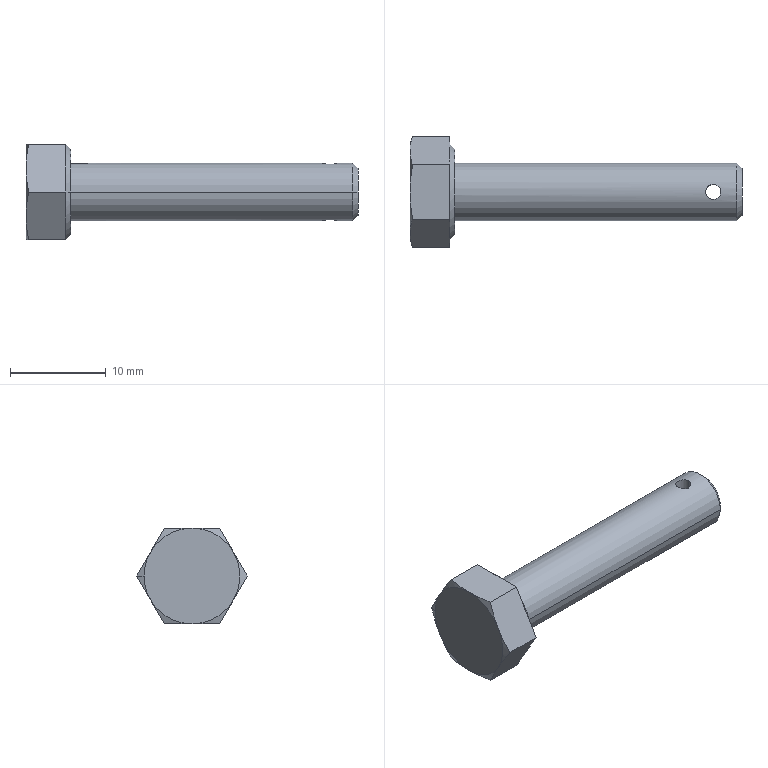Part | SolidWorks | features BaseBody 1 | 1 solid | 30 faces | box 34.65 x 11.547 x 10 mm | volume 1227 mm3 | plane 15 | cone 11 | cylinder 4 | commonest cylinder face diameters 1.6 x2 6 x2
STEP:
#1=CARTESIAN_POINT('',(30.85,0.,-3.));
#2=VERTEX_POINT('',#1);
#3=CARTESIAN_POINT('',(32.45,0.,-3.));
#4=VERTEX_POINT('',#3);
#5=CARTESIAN_POINT('',(30.85,0.,-3.));
#6=CARTESIAN_POINT('',(30.85,-0.1047,-3.));
#7=CARTESIAN_POINT('',(30.871,-0.2104,-2.994));
#8=CARTESIAN_POINT('',(30.951,-0.4032,-2.974));
#9=CARTESIAN_POINT('',(31.01,-0.4917,-2.96));
#10=CARTESIAN_POINT('',(31.232,-0.7131,-2.918));
#11=CARTESIAN_POINT('',(31.439,-0.7999,-2.891));
#12=CARTESIAN_POINT('',(31.755,-0.8,-2.891));
#13=CARTESIAN_POINT('',(31.86,-0.7789,-2.897));
#14=CARTESIAN_POINT('',(32.053,-0.6988,-2.918));
#15=CARTESIAN_POINT('',(32.142,-0.6393,-2.932));
#16=CARTESIAN_POINT('',(32.289,-0.4926,-2.96));
#17=CARTESIAN_POINT('',(32.348,-0.404,-2.974));
#18=CARTESIAN_POINT('',(32.429,-0.2113,-2.994));
#19=CARTESIAN_POINT('',(32.45,-0.1062,-3.));
#20=CARTESIAN_POINT('',(32.45,0.,-3.));
#21=B_SPLINE_CURVE_WITH_KNOTS('',3,(#5,#6,#7,#8,#9,#10,#11,#12,#13,#14,#15,#16,#17,#18,#19,#20),.UNSPECIFIED.,.F.,.F.,(4,2,2,2,2,2,2,4),(0.002513,0.002827,0.003141,0.003769,0.004083,0.004397,0.00471,0.005024),.UNSPECIFIED.);
#22=EDGE_CURVE('',#2,#4,#21,.T.);
#23=ORIENTED_EDGE('',*,*,#22,.F.);
#24=CARTESIAN_POINT('',(30.85,0.,3.));
#25=VERTEX_POINT('',#24);
#26=CARTESIAN_POINT('',(30.85,0.,-5.));
#27=DIRECTION('',(0.,0.,1.));
#28=VECTOR('',#27,1000.);
#29=LINE('',#26,#28);
#30=EDGE_CURVE('',#2,#25,#29,.T.);
#31=ORIENTED_EDGE('',*,*,#30,.T.);
#32=CARTESIAN_POINT('',(32.45,0.,3.));
#33=VERTEX_POINT('',#32);
#34=CARTESIAN_POINT('',(32.45,0.,3.));
#35=CARTESIAN_POINT('',(32.45,-0.1062,3.));
#36=CARTESIAN_POINT('',(32.429,-0.2104,2.994));
#37=CARTESIAN_POINT('',(32.348,-0.404,2.974));
#38=CARTESIAN_POINT('',(32.289,-0.4925,2.96));
#39=CARTESIAN_POINT('',(32.142,-0.6393,2.932));
#40=CARTESIAN_POINT('',(32.053,-0.6988,2.918));
#41=CARTESIAN_POINT('',(31.861,-0.7787,2.897));
#42=CARTESIAN_POINT('',(31.755,-0.8,2.891));
#43=CARTESIAN_POINT('',(31.545,-0.8,2.891));
#44=CARTESIAN_POINT('',(31.44,-0.7792,2.897));
#45=CARTESIAN_POINT('',(31.246,-0.6985,2.918));
#46=CARTESIAN_POINT('',(31.158,-0.6396,2.932));
#47=CARTESIAN_POINT('',(31.01,-0.4915,2.96));
#48=CARTESIAN_POINT('',(30.951,-0.4033,2.974));
#49=CARTESIAN_POINT('',(30.871,-0.2102,2.994));
#50=CARTESIAN_POINT('',(30.85,-0.1047,3.));
#51=CARTESIAN_POINT('',(30.85,0.,3.));
#52=B_SPLINE_CURVE_WITH_KNOTS('',3,(#34,#35,#36,#37,#38,#39,#40,#41,#42,#43,#44,#45,#46,#47,#48,#49,#50,#51),.UNSPECIFIED.,.F.,.F.,(4,2,2,2,2,2,2,2,4),(0.,0.0003141,0.0006281,0.0009422,0.001256,0.00157,0.001884,0.002199,0.002513),.UNSPECIFIED.);
#53=EDGE_CURVE('',#33,#25,#52,.T.);
#54=ORIENTED_EDGE('',*,*,#53,.F.);
#55=CARTESIAN_POINT('',(32.45,0.,-5.));
#56=DIRECTION('',(0.,0.,1.));
#57=VECTOR('',#56,1000.);
#58=LINE('',#55,#57);
#59=EDGE_CURVE('',#4,#33,#58,.T.);
#60=ORIENTED_EDGE('',*,*,#59,.F.);
#61=EDGE_LOOP('',(#23,#31,#54,#60));
#62=FACE_OUTER_BOUND('',#61,.T.);
#63=CARTESIAN_POINT('',(31.65,0.,-5.));
#64=DIRECTION('',(0.,0.,1.));
#65=DIRECTION('',(1.,0.,0.));
#66=AXIS2_PLACEMENT_3D('',#63,#64,#65);
#67=CYLINDRICAL_SURFACE('',#66,0.8);
#68=ADVANCED_FACE('',(#62),#67,.F.);
#69=CARTESIAN_POINT('',(34.65,2.459,0.));
#70=VERTEX_POINT('',#69);
#71=CARTESIAN_POINT('',(34.65,-2.458,0.));
#72=VERTEX_POINT('',#71);
#73=CARTESIAN_POINT('',(34.65,0.,0.));
#74=DIRECTION('',(1.,0.,0.));
#75=DIRECTION('',(0.,1.,0.));
#76=AXIS2_PLACEMENT_3D('',#73,#74,#75);
#77=CIRCLE('',#76,2.459);
#78=EDGE_CURVE('',#70,#72,#77,.T.);
#79=ORIENTED_EDGE('',*,*,#78,.F.);
#80=CARTESIAN_POINT('',(34.108,3.,0.));
#81=VERTEX_POINT('',#80);
#82=CARTESIAN_POINT('',(34.65,2.459,0.));
#83=DIRECTION('',(-0.7071,0.7071,0.));
#84=VECTOR('',#83,1000.);
#85=LINE('',#82,#84);
#86=EDGE_CURVE('',#70,#81,#85,.T.);
#87=ORIENTED_EDGE('',*,*,#86,.T.);
#88=CARTESIAN_POINT('',(34.108,-3.,0.));
#89=VERTEX_POINT('',#88);
#90=CARTESIAN_POINT('',(34.108,0.,0.));
#91=DIRECTION('',(-1.,0.,0.));
#92=DIRECTION('',(0.,1.,0.));
#93=AXIS2_PLACEMENT_3D('',#90,#91,#92);
#94=CIRCLE('',#93,3.);
#95=EDGE_CURVE('',#89,#81,#94,.T.);
#96=ORIENTED_EDGE('',*,*,#95,.F.);
#97=CARTESIAN_POINT('',(34.65,-2.458,0.));
#98=DIRECTION('',(-0.7071,-0.7071,0.));
#99=VECTOR('',#98,1000.);
#100=LINE('',#97,#99);
#101=EDGE_CURVE('',#72,#89,#100,.T.);
#102=ORIENTED_EDGE('',*,*,#101,.F.);
#103=EDGE_LOOP('',(#79,#87,#96,#102));
#104=FACE_OUTER_BOUND('',#103,.T.);
#105=CARTESIAN_POINT('',(34.65,0.,0.));
#106=DIRECTION('',(-1.,0.,0.));
#107=DIRECTION('',(0.,-1.,0.));
#108=AXIS2_PLACEMENT_3D('',#105,#106,#107);
#109=CONICAL_SURFACE('',#108,2.459,0.7854);
#110=ADVANCED_FACE('',(#104),#109,.T.);
#111=ORIENTED_EDGE('',*,*,#53,.T.);
#112=CARTESIAN_POINT('',(30.85,0.,3.));
#113=CARTESIAN_POINT('',(30.85,0.1047,3.));
#114=CARTESIAN_POINT('',(30.871,0.2104,2.994));
#115=CARTESIAN_POINT('',(30.951,0.4032,2.974));
#116=CARTESIAN_POINT('',(31.01,0.4917,2.96));
#117=CARTESIAN_POINT('',(31.232,0.7131,2.918));
#118=CARTESIAN_POINT('',(31.439,0.7999,2.891));
#119=CARTESIAN_POINT('',(31.755,0.8,2.891));
#120=CARTESIAN_POINT('',(31.86,0.7789,2.897));
#121=CARTESIAN_POINT('',(32.053,0.6988,2.918));
#122=CARTESIAN_POINT('',(32.142,0.6393,2.932));
#123=CARTESIAN_POINT('',(32.289,0.4926,2.96));
#124=CARTESIAN_POINT('',(32.348,0.404,2.974));
#125=CARTESIAN_POINT('',(32.429,0.2113,2.994));
#126=CARTESIAN_POINT('',(32.45,0.1062,3.));
#127=CARTESIAN_POINT('',(32.45,0.,3.));
#128=B_SPLINE_CURVE_WITH_KNOTS('',3,(#112,#113,#114,#115,#116,#117,#118,#119,#120,#121,#122,#123,#124,#125,#126,#127),.UNSPECIFIED.,.F.,.F.,(4,2,2,2,2,2,2,4),(0.002513,0.002827,0.003141,0.003769,0.004083,0.004397,0.00471,0.005024),.UNSPECIFIED.);
#129=EDGE_CURVE('',#25,#33,#128,.T.);
#130=ORIENTED_EDGE('',*,*,#129,.T.);
#131=EDGE_LOOP('',(#111,#130));
#132=FACE_BOUND('',#131,.T.);
#133=ORIENTED_EDGE('',*,*,#95,.T.);
#134=CARTESIAN_POINT('',(4.65,3.,0.));
#135=VERTEX_POINT('',#134);
#136=CARTESIAN_POINT('',(34.65,3.,0.));
#137=DIRECTION('',(-1.,0.,0.));
#138=VECTOR('',#137,1000.);
#139=LINE('',#136,#138);
#140=EDGE_CURVE('',#81,#135,#139,.T.);
#141=ORIENTED_EDGE('',*,*,#140,.T.);
#142=CARTESIAN_POINT('',(4.65,-3.,0.));
#143=VERTEX_POINT('',#142);
#144=CARTESIAN_POINT('',(4.65,0.,0.));
#145=DIRECTION('',(1.,0.,0.));
#146=DIRECTION('',(0.,-1.,0.));
#147=AXIS2_PLACEMENT_3D('',#144,#145,#146);
#148=CIRCLE('',#147,3.);
#149=EDGE_CURVE('',#135,#143,#148,.T.);
#150=ORIENTED_EDGE('',*,*,#149,.T.);
#151=CARTESIAN_POINT('',(34.65,-3.,0.));
#152=DIRECTION('',(-1.,0.,0.));
#153=VECTOR('',#152,1000.);
#154=LINE('',#151,#153);
#155=EDGE_CURVE('',#89,#143,#154,.T.);
#156=ORIENTED_EDGE('',*,*,#155,.F.);
#157=EDGE_LOOP('',(#133,#141,#150,#156));
#158=FACE_OUTER_BOUND('',#157,.T.);
#159=CARTESIAN_POINT('',(34.65,0.,0.));
#160=DIRECTION('',(-1.,0.,0.));
#161=DIRECTION('',(0.,-1.,0.));
#162=AXIS2_PLACEMENT_3D('',#159,#160,#161);
#163=CYLINDRICAL_SURFACE('',#162,3.);
#164=ADVANCED_FACE('',(#132,#158),#163,.T.);
#165=CARTESIAN_POINT('',(4.65,-4.45,0.));
#166=VERTEX_POINT('',#165);
#167=CARTESIAN_POINT('',(4.65,4.45,0.));
#168=VERTEX_POINT('',#167);
#169=CARTESIAN_POINT('',(4.65,0.,0.));
#170=DIRECTION('',(-1.,0.,0.));
#171=DIRECTION('',(0.,-1.,0.));
#172=AXIS2_PLACEMENT_3D('',#169,#170,#171);
#173=CIRCLE('',#172,4.45);
#174=EDGE_CURVE('',#166,#168,#173,.T.);
#175=ORIENTED_EDGE('',*,*,#174,.T.);
#176=CARTESIAN_POINT('',(4.15,5.,0.));
#177=VERTEX_POINT('',#176);
#178=CARTESIAN_POINT('',(4.65,4.45,0.));
#179=DIRECTION('',(-0.6727,0.7399,0.));
#180=VECTOR('',#179,1000.);
#181=LINE('',#178,#180);
#182=EDGE_CURVE('',#168,#177,#181,.T.);
#183=ORIENTED_EDGE('',*,*,#182,.T.);
#184=CARTESIAN_POINT('',(4.15,4.33,2.5));
#185=VERTEX_POINT('',#184);
#186=CARTESIAN_POINT('',(4.15,0.,0.));
#187=DIRECTION('',(-1.,0.,0.));
#188=DIRECTION('',(0.,-1.,0.));
#189=AXIS2_PLACEMENT_3D('',#186,#187,#188);
#190=CIRCLE('',#189,5.);
#191=EDGE_CURVE('',#185,#177,#190,.T.);
#192=ORIENTED_EDGE('',*,*,#191,.F.);
#193=CARTESIAN_POINT('',(4.15,0.,5.));
#194=VERTEX_POINT('',#193);
#195=CARTESIAN_POINT('',(4.15,0.,0.));
#196=DIRECTION('',(-1.,0.,0.));
#197=DIRECTION('',(0.,-1.,0.));
#198=AXIS2_PLACEMENT_3D('',#195,#196,#197);
#199=CIRCLE('',#198,5.);
#200=EDGE_CURVE('',#194,#185,#199,.T.);
#201=ORIENTED_EDGE('',*,*,#200,.F.);
#202=CARTESIAN_POINT('',(4.15,-4.33,2.5));
#203=VERTEX_POINT('',#202);
#204=CARTESIAN_POINT('',(4.15,0.,0.));
#205=DIRECTION('',(-1.,0.,0.));
#206=DIRECTION('',(0.,-1.,0.));
#207=AXIS2_PLACEMENT_3D('',#204,#205,#206);
#208=CIRCLE('',#207,5.);
#209=EDGE_CURVE('',#203,#194,#208,.T.);
#210=ORIENTED_EDGE('',*,*,#209,.F.);
#211=CARTESIAN_POINT('',(4.15,-5.,0.));
#212=VERTEX_POINT('',#211);
#213=CARTESIAN_POINT('',(4.15,0.,0.));
#214=DIRECTION('',(-1.,0.,0.));
#215=DIRECTION('',(0.,-1.,0.));
#216=AXIS2_PLACEMENT_3D('',#213,#214,#215);
#217=CIRCLE('',#216,5.);
#218=EDGE_CURVE('',#212,#203,#217,.T.);
#219=ORIENTED_EDGE('',*,*,#218,.F.);
#220=CARTESIAN_POINT('',(4.65,-4.45,0.));
#221=DIRECTION('',(-0.6727,-0.7399,0.));
#222=VECTOR('',#221,1000.);
#223=LINE('',#220,#222);
#224=EDGE_CURVE('',#166,#212,#223,.T.);
#225=ORIENTED_EDGE('',*,*,#224,.F.);
#226=EDGE_LOOP('',(#175,#183,#192,#201,#210,#219,#225));
#227=FACE_OUTER_BOUND('',#226,.T.);
#228=CARTESIAN_POINT('',(4.65,0.,0.));
#229=DIRECTION('',(-1.,0.,0.));
#230=DIRECTION('',(0.,-1.,0.));
#231=AXIS2_PLACEMENT_3D('',#228,#229,#230);
#232=CONICAL_SURFACE('',#231,4.45,0.833);
#233=ADVANCED_FACE('',(#227),#232,.T.);
#234=CARTESIAN_POINT('',(0.,4.33,-2.5));
#235=VERTEX_POINT('',#234);
#236=CARTESIAN_POINT('',(0.,5.,0.));
#237=VERTEX_POINT('',#236);
#238=CARTESIAN_POINT('',(0.,0.,0.));
#239=DIRECTION('',(1.,0.,0.));
#240=DIRECTION('',(0.,0.,-1.));
#241=AXIS2_PLACEMENT_3D('',#238,#239,#240);
#242=CIRCLE('',#241,5.);
#243=EDGE_CURVE('',#235,#237,#242,.T.);
#244=ORIENTED_EDGE('',*,*,#243,.T.);
#245=CARTESIAN_POINT('',(0.2815,5.774,0.));
#246=VERTEX_POINT('',#245);
#247=CARTESIAN_POINT('',(0.,5.,0.));
#248=DIRECTION('',(0.342,0.9397,0.));
#249=VECTOR('',#248,1000.);
#250=LINE('',#247,#249);
#251=EDGE_CURVE('',#237,#246,#250,.T.);
#252=ORIENTED_EDGE('',*,*,#251,.T.);
#253=CARTESIAN_POINT('',(0.2815,5.774,0.));
#254=CARTESIAN_POINT('',(0.1064,5.292,-0.8333));
#255=CARTESIAN_POINT('',(0.,4.811,-1.667));
#256=CARTESIAN_POINT('',(0.,4.33,-2.5));
#257=B_SPLINE_CURVE_WITH_KNOTS('',3,(#253,#254,#255,#256),.UNSPECIFIED.,.F.,.F.,(4,4),(0.000000231,0.002887),.UNSPECIFIED.);
#258=EDGE_CURVE('',#246,#235,#257,.T.);
#259=ORIENTED_EDGE('',*,*,#258,.T.);
#260=EDGE_LOOP('',(#244,#252,#259));
#261=FACE_OUTER_BOUND('',#260,.T.);
#262=CARTESIAN_POINT('',(0.,0.,0.));
#263=DIRECTION('',(1.,0.,0.));
#264=DIRECTION('',(0.,1.,0.));
#265=AXIS2_PLACEMENT_3D('',#262,#263,#264);
#266=CONICAL_SURFACE('',#265,5.,1.222);
#267=ADVANCED_FACE('',(#261),#266,.T.);
#268=ORIENTED_EDGE('',*,*,#174,.F.);
#269=CARTESIAN_POINT('',(4.65,0.,0.));
#270=DIRECTION('',(-1.,0.,0.));
#271=DIRECTION('',(0.,-1.,0.));
#272=AXIS2_PLACEMENT_3D('',#269,#270,#271);
#273=CIRCLE('',#272,4.45);
#274=EDGE_CURVE('',#168,#166,#273,.T.);
#275=ORIENTED_EDGE('',*,*,#274,.F.);
#276=EDGE_LOOP('',(#268,#275));
#277=FACE_OUTER_BOUND('',#276,.T.);
#278=CARTESIAN_POINT('',(4.65,0.,0.));
#279=DIRECTION('',(1.,0.,0.));
#280=DIRECTION('',(0.,-1.,0.));
#281=AXIS2_PLACEMENT_3D('',#278,#279,#280);
#282=CIRCLE('',#281,3.);
#283=EDGE_CURVE('',#143,#135,#282,.T.);
#284=ORIENTED_EDGE('',*,*,#283,.F.);
#285=ORIENTED_EDGE('',*,*,#149,.F.);
#286=EDGE_LOOP('',(#284,#285));
#287=FACE_BOUND('',#286,.T.);
#288=CARTESIAN_POINT('',(4.65,0.,0.));
#289=DIRECTION('',(-1.,0.,0.));
#290=DIRECTION('',(0.,-1.,0.));
#291=AXIS2_PLACEMENT_3D('',#288,#289,#290);
#292=PLANE('',#291);
#293=ADVANCED_FACE('',(#277,#287),#292,.F.);
#294=CARTESIAN_POINT('',(4.15,-2.887,5.));
#295=VERTEX_POINT('',#294);
#296=CARTESIAN_POINT('',(4.15,-2.887,5.));
#297=DIRECTION('',(0.,-0.5,-0.866));
#298=VECTOR('',#297,1000.);
#299=LINE('',#296,#298);
#300=EDGE_CURVE('',#295,#203,#299,.T.);
#301=ORIENTED_EDGE('',*,*,#300,.T.);
#302=ORIENTED_EDGE('',*,*,#209,.T.);
#303=CARTESIAN_POINT('',(4.15,2.887,5.));
#304=DIRECTION('',(0.,-1.,0.));
#305=VECTOR('',#304,1000.);
#306=LINE('',#303,#305);
#307=EDGE_CURVE('',#194,#295,#306,.T.);
#308=ORIENTED_EDGE('',*,*,#307,.T.);
#309=EDGE_LOOP('',(#301,#302,#308));
#310=FACE_OUTER_BOUND('',#309,.T.);
#311=CARTESIAN_POINT('',(4.15,-8.66,-5.));
#312=DIRECTION('',(1.,0.,0.));
#313=DIRECTION('',(0.,0.,-1.));
#314=AXIS2_PLACEMENT_3D('',#311,#312,#313);
#315=PLANE('',#314);
#316=ADVANCED_FACE('',(#310),#315,.T.);
#317=CARTESIAN_POINT('',(4.15,2.887,5.));
#318=VERTEX_POINT('',#317);
#319=CARTESIAN_POINT('',(4.15,2.887,5.));
#320=DIRECTION('',(0.,-1.,0.));
#321=VECTOR('',#320,1000.);
#322=LINE('',#319,#321);
#323=EDGE_CURVE('',#318,#194,#322,.T.);
#324=ORIENTED_EDGE('',*,*,#323,.T.);
#325=ORIENTED_EDGE('',*,*,#200,.T.);
#326=CARTESIAN_POINT('',(4.15,5.774,0.));
#327=DIRECTION('',(0.,-0.5,0.866));
#328=VECTOR('',#327,1000.);
#329=LINE('',#326,#328);
#330=EDGE_CURVE('',#185,#318,#329,.T.);
#331=ORIENTED_EDGE('',*,*,#330,.T.);
#332=EDGE_LOOP('',(#324,#325,#331));
#333=FACE_OUTER_BOUND('',#332,.T.);
#334=CARTESIAN_POINT('',(4.15,-8.66,-5.));
#335=DIRECTION('',(1.,0.,0.));
#336=DIRECTION('',(0.,0.,-1.));
#337=AXIS2_PLACEMENT_3D('',#334,#335,#336);
#338=PLANE('',#337);
#339=ADVANCED_FACE('',(#333),#338,.T.);
#340=CARTESIAN_POINT('',(4.15,5.774,0.));
#341=VERTEX_POINT('',#340);
#342=CARTESIAN_POINT('',(4.15,5.774,0.));
#343=DIRECTION('',(0.,-0.5,0.866));
#344=VECTOR('',#343,1000.);
#345=LINE('',#342,#344);
#346=EDGE_CURVE('',#341,#185,#345,.T.);
#347=ORIENTED_EDGE('',*,*,#346,.T.);
#348=ORIENTED_EDGE('',*,*,#191,.T.);
#349=CARTESIAN_POINT('',(4.15,4.33,-2.5));
#350=VERTEX_POINT('',#349);
#351=CARTESIAN_POINT('',(4.15,0.,0.));
#352=DIRECTION('',(-1.,0.,0.));
#353=DIRECTION('',(0.,-1.,0.));
#354=AXIS2_PLACEMENT_3D('',#351,#352,#353);
#355=CIRCLE('',#354,5.);
#356=EDGE_CURVE('',#177,#350,#355,.T.);
#357=ORIENTED_EDGE('',*,*,#356,.T.);
#358=CARTESIAN_POINT('',(4.15,2.887,-5.));
#359=DIRECTION('',(0.,0.5,0.866));
#360=VECTOR('',#359,1000.);
#361=LINE('',#358,#360);
#362=EDGE_CURVE('',#350,#341,#361,.T.);
#363=ORIENTED_EDGE('',*,*,#362,.T.);
#364=EDGE_LOOP('',(#347,#348,#357,#363));
#365=FACE_OUTER_BOUND('',#364,.T.);
#366=CARTESIAN_POINT('',(4.15,-8.66,-5.));
#367=DIRECTION('',(1.,0.,0.));
#368=DIRECTION('',(0.,0.,-1.));
#369=AXIS2_PLACEMENT_3D('',#366,#367,#368);
#370=PLANE('',#369);
#371=ADVANCED_FACE('',(#365),#370,.T.);
#372=CARTESIAN_POINT('',(4.15,2.887,-5.));
#373=VERTEX_POINT('',#372);
#374=CARTESIAN_POINT('',(4.15,2.887,-5.));
#375=DIRECTION('',(0.,0.5,0.866));
#376=VECTOR('',#375,1000.);
#377=LINE('',#374,#376);
#378=EDGE_CURVE('',#373,#350,#377,.T.);
#379=ORIENTED_EDGE('',*,*,#378,.T.);
#380=CARTESIAN_POINT('',(4.15,0.,-5.));
#381=VERTEX_POINT('',#380);
#382=CARTESIAN_POINT('',(4.15,0.,0.));
#383=DIRECTION('',(-1.,0.,0.));
#384=DIRECTION('',(0.,-1.,0.));
#385=AXIS2_PLACEMENT_3D('',#382,#383,#384);
#386=CIRCLE('',#385,5.);
#387=EDGE_CURVE('',#350,#381,#386,.T.);
#388=ORIENTED_EDGE('',*,*,#387,.T.);
#389=CARTESIAN_POINT('',(4.15,-2.887,-5.));
#390=DIRECTION('',(0.,1.,0.));
#391=VECTOR('',#390,1000.);
#392=LINE('',#389,#391);
#393=EDGE_CURVE('',#381,#373,#392,.T.);
#394=ORIENTED_EDGE('',*,*,#393,.T.);
#395=EDGE_LOOP('',(#379,#388,#394));
#396=FACE_OUTER_BOUND('',#395,.T.);
#397=CARTESIAN_POINT('',(4.15,-8.66,-5.));
#398=DIRECTION('',(1.,0.,0.));
#399=DIRECTION('',(0.,0.,-1.));
#400=AXIS2_PLACEMENT_3D('',#397,#398,#399);
#401=PLANE('',#400);
#402=ADVANCED_FACE('',(#396),#401,.T.);
#403=CARTESIAN_POINT('',(4.15,-2.887,-5.));
#404=VERTEX_POINT('',#403);
#405=CARTESIAN_POINT('',(4.15,-2.887,-5.));
#406=DIRECTION('',(0.,1.,0.));
#407=VECTOR('',#406,1000.);
#408=LINE('',#405,#407);
#409=EDGE_CURVE('',#404,#381,#408,.T.);
#410=ORIENTED_EDGE('',*,*,#409,.T.);
#411=CARTESIAN_POINT('',(4.15,-4.33,-2.5));
#412=VERTEX_POINT('',#411);
#413=CARTESIAN_POINT('',(4.15,0.,0.));
#414=DIRECTION('',(-1.,0.,0.));
#415=DIRECTION('',(0.,-1.,0.));
#416=AXIS2_PLACEMENT_3D('',#413,#414,#415);
#417=CIRCLE('',#416,5.);
#418=EDGE_CURVE('',#381,#412,#417,.T.);
#419=ORIENTED_EDGE('',*,*,#418,.T.);
#420=CARTESIAN_POINT('',(4.15,-5.774,0.));
#421=DIRECTION('',(0.,0.5,-0.866));
#422=VECTOR('',#421,1000.);
#423=LINE('',#420,#422);
#424=EDGE_CURVE('',#412,#404,#423,.T.);
#425=ORIENTED_EDGE('',*,*,#424,.T.);
#426=EDGE_LOOP('',(#410,#419,#425));
#427=FACE_OUTER_BOUND('',#426,.T.);
#428=CARTESIAN_POINT('',(4.15,-8.66,-5.));
#429=DIRECTION('',(1.,0.,0.));
#430=DIRECTION('',(0.,0.,-1.));
#431=AXIS2_PLACEMENT_3D('',#428,#429,#430);
#432=PLANE('',#431);
#433=ADVANCED_FACE('',(#427),#432,.T.);
#434=CARTESIAN_POINT('',(4.15,-5.774,0.));
#435=VERTEX_POINT('',#434);
#436=CARTESIAN_POINT('',(4.15,-5.774,0.));
#437=DIRECTION('',(0.,0.5,-0.866));
#438=VECTOR('',#437,1000.);
#439=LINE('',#436,#438);
#440=EDGE_CURVE('',#435,#412,#439,.T.);
#441=ORIENTED_EDGE('',*,*,#440,.T.);
#442=CARTESIAN_POINT('',(4.15,0.,0.));
#443=DIRECTION('',(-1.,0.,0.));
#444=DIRECTION('',(0.,-1.,0.));
#445=AXIS2_PLACEMENT_3D('',#442,#443,#444);
#446=CIRCLE('',#445,5.);
#447=EDGE_CURVE('',#412,#212,#446,.T.);
#448=ORIENTED_EDGE('',*,*,#447,.T.);
#449=ORIENTED_EDGE('',*,*,#218,.T.);
#450=CARTESIAN_POINT('',(4.15,-2.887,5.));
#451=DIRECTION('',(0.,-0.5,-0.866));
#452=VECTOR('',#451,1000.);
#453=LINE('',#450,#452);
#454=EDGE_CURVE('',#203,#435,#453,.T.);
#455=ORIENTED_EDGE('',*,*,#454,.T.);
#456=EDGE_LOOP('',(#441,#448,#449,#455));
#457=FACE_OUTER_BOUND('',#456,.T.);
#458=CARTESIAN_POINT('',(4.15,-8.66,-5.));
#459=DIRECTION('',(1.,0.,0.));
#460=DIRECTION('',(0.,0.,-1.));
#461=AXIS2_PLACEMENT_3D('',#458,#459,#460);
#462=PLANE('',#461);
#463=ADVANCED_FACE('',(#457),#462,.T.);
#464=CARTESIAN_POINT('',(0.2815,-5.774,0.));
#465=VERTEX_POINT('',#464);
#466=CARTESIAN_POINT('',(0.,-4.33,2.5));
#467=VERTEX_POINT('',#466);
#468=CARTESIAN_POINT('',(0.2815,-5.774,0.));
#469=CARTESIAN_POINT('',(0.1064,-5.292,0.8333));
#470=CARTESIAN_POINT('',(0.,-4.811,1.667));
#471=CARTESIAN_POINT('',(0.,-4.33,2.5));
#472=B_SPLINE_CURVE_WITH_KNOTS('',3,(#468,#469,#470,#471),.UNSPECIFIED.,.F.,.F.,(4,4),(0.000000231,0.002887),.UNSPECIFIED.);
#473=EDGE_CURVE('',#465,#467,#472,.T.);
#474=ORIENTED_EDGE('',*,*,#473,.F.);
#475=CARTESIAN_POINT('',(4.15,-5.774,0.));
#476=DIRECTION('',(-1.,0.,0.));
#477=VECTOR('',#476,1000.);
#478=LINE('',#475,#477);
#479=EDGE_CURVE('',#435,#465,#478,.T.);
#480=ORIENTED_EDGE('',*,*,#479,.F.);
#481=ORIENTED_EDGE('',*,*,#454,.F.);
#482=ORIENTED_EDGE('',*,*,#300,.F.);
#483=CARTESIAN_POINT('',(0.2815,-2.887,5.));
#484=VERTEX_POINT('',#483);
#485=CARTESIAN_POINT('',(4.15,-2.887,5.));
#486=DIRECTION('',(-1.,0.,0.));
#487=VECTOR('',#486,1000.);
#488=LINE('',#485,#487);
#489=EDGE_CURVE('',#295,#484,#488,.T.);
#490=ORIENTED_EDGE('',*,*,#489,.T.);
#491=CARTESIAN_POINT('',(0.,-4.33,2.5));
#492=CARTESIAN_POINT('',(0.,-3.849,3.333));
#493=CARTESIAN_POINT('',(0.1064,-3.368,4.167));
#494=CARTESIAN_POINT('',(0.2815,-2.887,5.));
#495=B_SPLINE_CURVE_WITH_KNOTS('',3,(#491,#492,#493,#494),.UNSPECIFIED.,.F.,.F.,(4,4),(0.002887,0.005774),.UNSPECIFIED.);
#496=EDGE_CURVE('',#467,#484,#495,.T.);
#497=ORIENTED_EDGE('',*,*,#496,.F.);
#498=EDGE_LOOP('',(#474,#480,#481,#482,#490,#497));
#499=FACE_OUTER_BOUND('',#498,.T.);
#500=CARTESIAN_POINT('',(4.15,-2.887,5.));
#501=DIRECTION('',(0.,0.866,-0.5));
#502=DIRECTION('',(0.,0.5,0.866));
#503=AXIS2_PLACEMENT_3D('',#500,#501,#502);
#504=PLANE('',#503);
#505=ADVANCED_FACE('',(#499),#504,.F.);
#506=CARTESIAN_POINT('',(0.2815,-2.887,-5.));
#507=VERTEX_POINT('',#506);
#508=CARTESIAN_POINT('',(0.,-4.33,-2.5));
#509=VERTEX_POINT('',#508);
#510=CARTESIAN_POINT('',(0.2815,-2.887,-5.));
#511=CARTESIAN_POINT('',(0.1064,-3.368,-4.167));
#512=CARTESIAN_POINT('',(0.,-3.849,-3.333));
#513=CARTESIAN_POINT('',(0.,-4.33,-2.5));
#514=B_SPLINE_CURVE_WITH_KNOTS('',3,(#510,#511,#512,#513),.UNSPECIFIED.,.F.,.F.,(4,4),(0.000000231,0.002887),.UNSPECIFIED.);
#515=EDGE_CURVE('',#507,#509,#514,.T.);
#516=ORIENTED_EDGE('',*,*,#515,.F.);
#517=CARTESIAN_POINT('',(4.15,-2.887,-5.));
#518=DIRECTION('',(-1.,0.,0.));
#519=VECTOR('',#518,1000.);
#520=LINE('',#517,#519);
#521=EDGE_CURVE('',#404,#507,#520,.T.);
#522=ORIENTED_EDGE('',*,*,#521,.F.);
#523=ORIENTED_EDGE('',*,*,#424,.F.);
#524=ORIENTED_EDGE('',*,*,#440,.F.);
#525=ORIENTED_EDGE('',*,*,#479,.T.);
#526=CARTESIAN_POINT('',(0.,-4.33,-2.5));
#527=CARTESIAN_POINT('',(0.,-4.811,-1.667));
#528=CARTESIAN_POINT('',(0.1064,-5.292,-0.8333));
#529=CARTESIAN_POINT('',(0.2815,-5.774,0.));
#530=B_SPLINE_CURVE_WITH_KNOTS('',3,(#526,#527,#528,#529),.UNSPECIFIED.,.F.,.F.,(4,4),(0.002887,0.005774),.UNSPECIFIED.);
#531=EDGE_CURVE('',#509,#465,#530,.T.);
#532=ORIENTED_EDGE('',*,*,#531,.F.);
#533=EDGE_LOOP('',(#516,#522,#523,#524,#525,#532));
#534=FACE_OUTER_BOUND('',#533,.T.);
#535=CARTESIAN_POINT('',(4.15,-5.774,0.));
#536=DIRECTION('',(0.,0.866,0.5));
#537=DIRECTION('',(0.,-0.5,0.866));
#538=AXIS2_PLACEMENT_3D('',#535,#536,#537);
#539=PLANE('',#538);
#540=ADVANCED_FACE('',(#534),#539,.F.);
#541=CARTESIAN_POINT('',(0.2815,2.887,-5.));
#542=VERTEX_POINT('',#541);
#543=CARTESIAN_POINT('',(0.,0.,-5.));
#544=VERTEX_POINT('',#543);
#545=CARTESIAN_POINT('',(0.2815,2.887,-5.));
#546=CARTESIAN_POINT('',(0.1069,1.927,-5.));
#547=CARTESIAN_POINT('',(0.,0.9642,-5.));
#548=CARTESIAN_POINT('',(0.,0.,-5.));
#549=B_SPLINE_CURVE_WITH_KNOTS('',3,(#545,#546,#547,#548),.UNSPECIFIED.,.F.,.F.,(4,4),(0.01041,0.01332),.UNSPECIFIED.);
#550=EDGE_CURVE('',#542,#544,#549,.T.);
#551=ORIENTED_EDGE('',*,*,#550,.F.);
#552=CARTESIAN_POINT('',(4.15,2.887,-5.));
#553=DIRECTION('',(-1.,0.,0.));
#554=VECTOR('',#553,1000.);
#555=LINE('',#552,#554);
#556=EDGE_CURVE('',#373,#542,#555,.T.);
#557=ORIENTED_EDGE('',*,*,#556,.F.);
#558=ORIENTED_EDGE('',*,*,#393,.F.);
#559=ORIENTED_EDGE('',*,*,#409,.F.);
#560=ORIENTED_EDGE('',*,*,#521,.T.);
#561=CARTESIAN_POINT('',(0.,0.,-5.));
#562=CARTESIAN_POINT('',(0.,-0.4807,-5.));
#563=CARTESIAN_POINT('',(0.02571,-0.962,-5.));
#564=CARTESIAN_POINT('',(0.123,-1.926,-5.));
#565=CARTESIAN_POINT('',(0.1945,-2.409,-5.));
#566=CARTESIAN_POINT('',(0.2815,-2.887,-5.));
#567=B_SPLINE_CURVE_WITH_KNOTS('',3,(#561,#562,#563,#564,#565,#566),.UNSPECIFIED.,.F.,.F.,(4,2,4),(0.01332,0.01477,0.01622),.UNSPECIFIED.);
#568=EDGE_CURVE('',#544,#507,#567,.T.);
#569=ORIENTED_EDGE('',*,*,#568,.F.);
#570=EDGE_LOOP('',(#551,#557,#558,#559,#560,#569));
#571=FACE_OUTER_BOUND('',#570,.T.);
#572=CARTESIAN_POINT('',(4.15,-2.887,-5.));
#573=DIRECTION('',(0.,0.,1.));
#574=DIRECTION('',(1.,0.,0.));
#575=AXIS2_PLACEMENT_3D('',#572,#573,#574);
#576=PLANE('',#575);
#577=ADVANCED_FACE('',(#571),#576,.F.);
#578=ORIENTED_EDGE('',*,*,#258,.F.);
#579=CARTESIAN_POINT('',(4.15,5.774,0.));
#580=DIRECTION('',(-1.,0.,0.));
#581=VECTOR('',#580,1000.);
#582=LINE('',#579,#581);
#583=EDGE_CURVE('',#341,#246,#582,.T.);
#584=ORIENTED_EDGE('',*,*,#583,.F.);
#585=ORIENTED_EDGE('',*,*,#362,.F.);
#586=ORIENTED_EDGE('',*,*,#378,.F.);
#587=ORIENTED_EDGE('',*,*,#556,.T.);
#588=CARTESIAN_POINT('',(0.,4.33,-2.5));
#589=CARTESIAN_POINT('',(0.,3.849,-3.333));
#590=CARTESIAN_POINT('',(0.1064,3.368,-4.167));
#591=CARTESIAN_POINT('',(0.2815,2.887,-5.));
#592=B_SPLINE_CURVE_WITH_KNOTS('',3,(#588,#589,#590,#591),.UNSPECIFIED.,.F.,.F.,(4,4),(0.002887,0.005774),.UNSPECIFIED.);
#593=EDGE_CURVE('',#235,#542,#592,.T.);
#594=ORIENTED_EDGE('',*,*,#593,.F.);
#595=EDGE_LOOP('',(#578,#584,#585,#586,#587,#594));
#596=FACE_OUTER_BOUND('',#595,.T.);
#597=CARTESIAN_POINT('',(4.15,2.887,-5.));
#598=DIRECTION('',(0.,-0.866,0.5));
#599=DIRECTION('',(0.,-0.5,-0.866));
#600=AXIS2_PLACEMENT_3D('',#597,#598,#599);
#601=PLANE('',#600);
#602=ADVANCED_FACE('',(#596),#601,.F.);
#603=CARTESIAN_POINT('',(0.2815,2.887,5.));
#604=VERTEX_POINT('',#603);
#605=CARTESIAN_POINT('',(0.,4.33,2.5));
#606=VERTEX_POINT('',#605);
#607=CARTESIAN_POINT('',(0.2815,2.887,5.));
#608=CARTESIAN_POINT('',(0.1064,3.368,4.167));
#609=CARTESIAN_POINT('',(0.,3.849,3.333));
#610=CARTESIAN_POINT('',(0.,4.33,2.5));
#611=B_SPLINE_CURVE_WITH_KNOTS('',3,(#607,#608,#609,#610),.UNSPECIFIED.,.F.,.F.,(4,4),(0.000000231,0.002887),.UNSPECIFIED.);
#612=EDGE_CURVE('',#604,#606,#611,.T.);
#613=ORIENTED_EDGE('',*,*,#612,.F.);
#614=CARTESIAN_POINT('',(4.15,2.887,5.));
#615=DIRECTION('',(-1.,0.,0.));
#616=VECTOR('',#615,1000.);
#617=LINE('',#614,#616);
#618=EDGE_CURVE('',#318,#604,#617,.T.);
#619=ORIENTED_EDGE('',*,*,#618,.F.);
#620=ORIENTED_EDGE('',*,*,#330,.F.);
#621=ORIENTED_EDGE('',*,*,#346,.F.);
#622=ORIENTED_EDGE('',*,*,#583,.T.);
#623=CARTESIAN_POINT('',(0.,4.33,2.5));
#624=CARTESIAN_POINT('',(0.,4.811,1.667));
#625=CARTESIAN_POINT('',(0.1064,5.292,0.8333));
#626=CARTESIAN_POINT('',(0.2815,5.774,0.));
#627=B_SPLINE_CURVE_WITH_KNOTS('',3,(#623,#624,#625,#626),.UNSPECIFIED.,.F.,.F.,(4,4),(0.002887,0.005774),.UNSPECIFIED.);
#628=EDGE_CURVE('',#606,#246,#627,.T.);
#629=ORIENTED_EDGE('',*,*,#628,.F.);
#630=EDGE_LOOP('',(#613,#619,#620,#621,#622,#629));
#631=FACE_OUTER_BOUND('',#630,.T.);
#632=CARTESIAN_POINT('',(4.15,5.774,0.));
#633=DIRECTION('',(0.,-0.866,-0.5));
#634=DIRECTION('',(0.,0.5,-0.866));
#635=AXIS2_PLACEMENT_3D('',#632,#633,#634);
#636=PLANE('',#635);
#637=ADVANCED_FACE('',(#631),#636,.F.);
#638=CARTESIAN_POINT('',(0.,0.,5.));
#639=VERTEX_POINT('',#638);
#640=CARTESIAN_POINT('',(0.2815,-2.887,5.));
#641=CARTESIAN_POINT('',(0.1945,-2.409,5.));
#642=CARTESIAN_POINT('',(0.123,-1.926,5.));
#643=CARTESIAN_POINT('',(0.02571,-0.962,5.));
#644=CARTESIAN_POINT('',(0.,-0.4807,5.));
#645=CARTESIAN_POINT('',(0.,0.,5.));
#646=B_SPLINE_CURVE_WITH_KNOTS('',3,(#640,#641,#642,#643,#644,#645),.UNSPECIFIED.,.F.,.F.,(4,2,4),(0.004911,0.006366,0.00782),.UNSPECIFIED.);
#647=EDGE_CURVE('',#484,#639,#646,.T.);
#648=ORIENTED_EDGE('',*,*,#647,.F.);
#649=ORIENTED_EDGE('',*,*,#489,.F.);
#650=ORIENTED_EDGE('',*,*,#307,.F.);
#651=ORIENTED_EDGE('',*,*,#323,.F.);
#652=ORIENTED_EDGE('',*,*,#618,.T.);
#653=CARTESIAN_POINT('',(0.,0.,5.));
#654=CARTESIAN_POINT('',(0.,0.9642,5.));
#655=CARTESIAN_POINT('',(0.1069,1.927,5.));
#656=CARTESIAN_POINT('',(0.2815,2.887,5.));
#657=B_SPLINE_CURVE_WITH_KNOTS('',3,(#653,#654,#655,#656),.UNSPECIFIED.,.F.,.F.,(4,4),(0.00782,0.01074),.UNSPECIFIED.);
#658=EDGE_CURVE('',#639,#604,#657,.T.);
#659=ORIENTED_EDGE('',*,*,#658,.F.);
#660=EDGE_LOOP('',(#648,#649,#650,#651,#652,#659));
#661=FACE_OUTER_BOUND('',#660,.T.);
#662=CARTESIAN_POINT('',(4.15,2.887,5.));
#663=DIRECTION('',(0.,0.,-1.));
#664=DIRECTION('',(-1.,0.,0.));
#665=AXIS2_PLACEMENT_3D('',#662,#663,#664);
#666=PLANE('',#665);
#667=ADVANCED_FACE('',(#661),#666,.F.);
#668=ORIENTED_EDGE('',*,*,#568,.T.);
#669=ORIENTED_EDGE('',*,*,#515,.T.);
#670=CARTESIAN_POINT('',(0.,0.,0.));
#671=DIRECTION('',(1.,0.,0.));
#672=DIRECTION('',(0.,0.,-1.));
#673=AXIS2_PLACEMENT_3D('',#670,#671,#672);
#674=CIRCLE('',#673,5.);
#675=EDGE_CURVE('',#509,#544,#674,.T.);
#676=ORIENTED_EDGE('',*,*,#675,.T.);
#677=EDGE_LOOP('',(#668,#669,#676));
#678=FACE_OUTER_BOUND('',#677,.T.);
#679=CARTESIAN_POINT('',(0.,0.,0.));
#680=DIRECTION('',(1.,0.,0.));
#681=DIRECTION('',(0.,1.,0.));
#682=AXIS2_PLACEMENT_3D('',#679,#680,#681);
#683=CONICAL_SURFACE('',#682,5.,1.222);
#684=ADVANCED_FACE('',(#678),#683,.T.);
#685=ORIENTED_EDGE('',*,*,#531,.T.);
#686=ORIENTED_EDGE('',*,*,#473,.T.);
#687=CARTESIAN_POINT('',(0.,0.,0.));
#688=DIRECTION('',(1.,0.,0.));
#689=DIRECTION('',(0.,0.,-1.));
#690=AXIS2_PLACEMENT_3D('',#687,#688,#689);
#691=CIRCLE('',#690,5.);
#692=EDGE_CURVE('',#467,#509,#691,.T.);
#693=ORIENTED_EDGE('',*,*,#692,.T.);
#694=EDGE_LOOP('',(#685,#686,#693));
#695=FACE_OUTER_BOUND('',#694,.T.);
#696=CARTESIAN_POINT('',(0.,0.,0.));
#697=DIRECTION('',(1.,0.,0.));
#698=DIRECTION('',(0.,1.,0.));
#699=AXIS2_PLACEMENT_3D('',#696,#697,#698);
#700=CONICAL_SURFACE('',#699,5.,1.222);
#701=ADVANCED_FACE('',(#695),#700,.T.);
#702=ORIENTED_EDGE('',*,*,#496,.T.);
#703=ORIENTED_EDGE('',*,*,#647,.T.);
#704=CARTESIAN_POINT('',(0.,0.,0.));
#705=DIRECTION('',(-1.,0.,0.));
#706=DIRECTION('',(0.,-1.,0.));
#707=AXIS2_PLACEMENT_3D('',#704,#705,#706);
#708=CIRCLE('',#707,5.);
#709=EDGE_CURVE('',#467,#639,#708,.T.);
#710=ORIENTED_EDGE('',*,*,#709,.F.);
#711=EDGE_LOOP('',(#702,#703,#710));
#712=FACE_OUTER_BOUND('',#711,.T.);
#713=CARTESIAN_POINT('',(0.,0.,0.));
#714=DIRECTION('',(1.,0.,0.));
#715=DIRECTION('',(0.,1.,0.));
#716=AXIS2_PLACEMENT_3D('',#713,#714,#715);
#717=CONICAL_SURFACE('',#716,5.,1.222);
#718=ADVANCED_FACE('',(#712),#717,.T.);
#719=ORIENTED_EDGE('',*,*,#612,.T.);
#720=CARTESIAN_POINT('',(0.,0.,0.));
#721=DIRECTION('',(1.,0.,0.));
#722=DIRECTION('',(0.,0.,-1.));
#723=AXIS2_PLACEMENT_3D('',#720,#721,#722);
#724=CIRCLE('',#723,5.);
#725=EDGE_CURVE('',#606,#639,#724,.T.);
#726=ORIENTED_EDGE('',*,*,#725,.T.);
#727=ORIENTED_EDGE('',*,*,#658,.T.);
#728=EDGE_LOOP('',(#719,#726,#727));
#729=FACE_OUTER_BOUND('',#728,.T.);
#730=CARTESIAN_POINT('',(0.,0.,0.));
#731=DIRECTION('',(1.,0.,0.));
#732=DIRECTION('',(0.,1.,0.));
#733=AXIS2_PLACEMENT_3D('',#730,#731,#732);
#734=CONICAL_SURFACE('',#733,5.,1.222);
#735=ADVANCED_FACE('',(#729),#734,.T.);
#736=ORIENTED_EDGE('',*,*,#251,.F.);
#737=CARTESIAN_POINT('',(0.,0.,0.));
#738=DIRECTION('',(1.,0.,0.));
#739=DIRECTION('',(0.,0.,-1.));
#740=AXIS2_PLACEMENT_3D('',#737,#738,#739);
#741=CIRCLE('',#740,5.);
#742=EDGE_CURVE('',#237,#606,#741,.T.);
#743=ORIENTED_EDGE('',*,*,#742,.T.);
#744=ORIENTED_EDGE('',*,*,#628,.T.);
#745=EDGE_LOOP('',(#736,#743,#744));
#746=FACE_OUTER_BOUND('',#745,.T.);
#747=CARTESIAN_POINT('',(0.,0.,0.));
#748=DIRECTION('',(1.,0.,0.));
#749=DIRECTION('',(0.,1.,0.));
#750=AXIS2_PLACEMENT_3D('',#747,#748,#749);
#751=CONICAL_SURFACE('',#750,5.,1.222);
#752=ADVANCED_FACE('',(#746),#751,.T.);
#753=ORIENTED_EDGE('',*,*,#550,.T.);
#754=CARTESIAN_POINT('',(0.,0.,0.));
#755=DIRECTION('',(1.,0.,0.));
#756=DIRECTION('',(0.,0.,-1.));
#757=AXIS2_PLACEMENT_3D('',#754,#755,#756);
#758=CIRCLE('',#757,5.);
#759=EDGE_CURVE('',#544,#235,#758,.T.);
#760=ORIENTED_EDGE('',*,*,#759,.T.);
#761=ORIENTED_EDGE('',*,*,#593,.T.);
#762=EDGE_LOOP('',(#753,#760,#761));
#763=FACE_OUTER_BOUND('',#762,.T.);
#764=CARTESIAN_POINT('',(0.,0.,0.));
#765=DIRECTION('',(1.,0.,0.));
#766=DIRECTION('',(0.,1.,0.));
#767=AXIS2_PLACEMENT_3D('',#764,#765,#766);
#768=CONICAL_SURFACE('',#767,5.,1.222);
#769=ADVANCED_FACE('',(#763),#768,.T.);
#770=ORIENTED_EDGE('',*,*,#759,.F.);
#771=ORIENTED_EDGE('',*,*,#675,.F.);
#772=ORIENTED_EDGE('',*,*,#692,.F.);
#773=ORIENTED_EDGE('',*,*,#709,.T.);
#774=ORIENTED_EDGE('',*,*,#725,.F.);
#775=ORIENTED_EDGE('',*,*,#742,.F.);
#776=ORIENTED_EDGE('',*,*,#243,.F.);
#777=EDGE_LOOP('',(#770,#771,#772,#773,#774,#775,#776));
#778=FACE_OUTER_BOUND('',#777,.T.);
#779=CARTESIAN_POINT('',(0.,-8.66,-5.));
#780=DIRECTION('',(1.,0.,0.));
#781=DIRECTION('',(0.,0.,-1.));
#782=AXIS2_PLACEMENT_3D('',#779,#780,#781);
#783=PLANE('',#782);
#784=ADVANCED_FACE('',(#778),#783,.F.);
#785=ORIENTED_EDGE('',*,*,#182,.F.);
#786=ORIENTED_EDGE('',*,*,#274,.T.);
#787=ORIENTED_EDGE('',*,*,#224,.T.);
#788=ORIENTED_EDGE('',*,*,#447,.F.);
#789=ORIENTED_EDGE('',*,*,#418,.F.);
#790=ORIENTED_EDGE('',*,*,#387,.F.);
#791=ORIENTED_EDGE('',*,*,#356,.F.);
#792=EDGE_LOOP('',(#785,#786,#787,#788,#789,#790,#791));
#793=FACE_OUTER_BOUND('',#792,.T.);
#794=CARTESIAN_POINT('',(4.65,0.,0.));
#795=DIRECTION('',(-1.,0.,0.));
#796=DIRECTION('',(0.,-1.,0.));
#797=AXIS2_PLACEMENT_3D('',#794,#795,#796);
#798=CONICAL_SURFACE('',#797,4.45,0.833);
#799=ADVANCED_FACE('',(#793),#798,.T.);
#800=ORIENTED_EDGE('',*,*,#140,.F.);
#801=CARTESIAN_POINT('',(34.108,0.,0.));
#802=DIRECTION('',(-1.,0.,0.));
#803=DIRECTION('',(0.,1.,0.));
#804=AXIS2_PLACEMENT_3D('',#801,#802,#803);
#805=CIRCLE('',#804,3.);
#806=EDGE_CURVE('',#81,#89,#805,.T.);
#807=ORIENTED_EDGE('',*,*,#806,.T.);
#808=ORIENTED_EDGE('',*,*,#155,.T.);
#809=ORIENTED_EDGE('',*,*,#283,.T.);
#810=EDGE_LOOP('',(#800,#807,#808,#809));
#811=FACE_OUTER_BOUND('',#810,.T.);
#812=CARTESIAN_POINT('',(32.45,0.,-3.));
#813=CARTESIAN_POINT('',(32.45,0.1062,-3.));
#814=CARTESIAN_POINT('',(32.429,0.2104,-2.994));
#815=CARTESIAN_POINT('',(32.348,0.404,-2.974));
#816=CARTESIAN_POINT('',(32.289,0.4925,-2.96));
#817=CARTESIAN_POINT('',(32.142,0.6393,-2.932));
#818=CARTESIAN_POINT('',(32.053,0.6988,-2.918));
#819=CARTESIAN_POINT('',(31.861,0.7787,-2.897));
#820=CARTESIAN_POINT('',(31.755,0.8,-2.891));
#821=CARTESIAN_POINT('',(31.545,0.8,-2.891));
#822=CARTESIAN_POINT('',(31.44,0.7792,-2.897));
#823=CARTESIAN_POINT('',(31.246,0.6985,-2.918));
#824=CARTESIAN_POINT('',(31.158,0.6396,-2.932));
#825=CARTESIAN_POINT('',(31.01,0.4915,-2.96));
#826=CARTESIAN_POINT('',(30.951,0.4033,-2.974));
#827=CARTESIAN_POINT('',(30.871,0.2102,-2.994));
#828=CARTESIAN_POINT('',(30.85,0.1047,-3.));
#829=CARTESIAN_POINT('',(30.85,0.,-3.));
#830=B_SPLINE_CURVE_WITH_KNOTS('',3,(#812,#813,#814,#815,#816,#817,#818,#819,#820,#821,#822,#823,#824,#825,#826,#827,#828,#829),.UNSPECIFIED.,.F.,.F.,(4,2,2,2,2,2,2,2,4),(0.,0.0003141,0.0006281,0.0009422,0.001256,0.00157,0.001884,0.002199,0.002513),.UNSPECIFIED.);
#831=EDGE_CURVE('',#4,#2,#830,.T.);
#832=ORIENTED_EDGE('',*,*,#831,.T.);
#833=ORIENTED_EDGE('',*,*,#22,.T.);
#834=EDGE_LOOP('',(#832,#833));
#835=FACE_BOUND('',#834,.T.);
#836=CARTESIAN_POINT('',(34.65,0.,0.));
#837=DIRECTION('',(-1.,0.,0.));
#838=DIRECTION('',(0.,-1.,0.));
#839=AXIS2_PLACEMENT_3D('',#836,#837,#838);
#840=CYLINDRICAL_SURFACE('',#839,3.);
#841=ADVANCED_FACE('',(#811,#835),#840,.T.);
#842=CARTESIAN_POINT('',(34.65,0.,0.));
#843=DIRECTION('',(1.,0.,0.));
#844=DIRECTION('',(0.,1.,0.));
#845=AXIS2_PLACEMENT_3D('',#842,#843,#844);
#846=CIRCLE('',#845,2.459);
#847=EDGE_CURVE('',#72,#70,#846,.T.);
#848=ORIENTED_EDGE('',*,*,#847,.T.);
#849=ORIENTED_EDGE('',*,*,#78,.T.);
#850=EDGE_LOOP('',(#848,#849));
#851=FACE_OUTER_BOUND('',#850,.T.);
#852=CARTESIAN_POINT('',(34.65,0.,0.));
#853=DIRECTION('',(1.,0.,0.));
#854=DIRECTION('',(0.,1.,0.));
#855=AXIS2_PLACEMENT_3D('',#852,#853,#854);
#856=PLANE('',#855);
#857=ADVANCED_FACE('',(#851),#856,.T.);
#858=ORIENTED_EDGE('',*,*,#86,.F.);
#859=ORIENTED_EDGE('',*,*,#847,.F.);
#860=ORIENTED_EDGE('',*,*,#101,.T.);
#861=ORIENTED_EDGE('',*,*,#806,.F.);
#862=EDGE_LOOP('',(#858,#859,#860,#861));
#863=FACE_OUTER_BOUND('',#862,.T.);
#864=CARTESIAN_POINT('',(34.65,0.,0.));
#865=DIRECTION('',(-1.,0.,0.));
#866=DIRECTION('',(0.,-1.,0.));
#867=AXIS2_PLACEMENT_3D('',#864,#865,#866);
#868=CONICAL_SURFACE('',#867,2.459,0.7854);
#869=ADVANCED_FACE('',(#863),#868,.T.);
#870=ORIENTED_EDGE('',*,*,#30,.F.);
#871=ORIENTED_EDGE('',*,*,#831,.F.);
#872=ORIENTED_EDGE('',*,*,#59,.T.);
#873=ORIENTED_EDGE('',*,*,#129,.F.);
#874=EDGE_LOOP('',(#870,#871,#872,#873));
#875=FACE_OUTER_BOUND('',#874,.T.);
#876=CARTESIAN_POINT('',(31.65,0.,-5.));
#877=DIRECTION('',(0.,0.,1.));
#878=DIRECTION('',(1.,0.,0.));
#879=AXIS2_PLACEMENT_3D('',#876,#877,#878);
#880=CYLINDRICAL_SURFACE('',#879,0.8);
#881=ADVANCED_FACE('',(#875),#880,.F.);
#882=CLOSED_SHELL('',(#68,#110,#164,#233,#267,#293,#316,#339,#371,#402,#433,#463,#505,#540,#577,#602,#637,#667,#684,#701,#718,#735,#752,#769,#784,#799,#841,#857,#869,#881));
#883=MANIFOLD_SOLID_BREP('',#882);
#884=CARTESIAN_POINT('',(0.,0.,0.));
#885=DIRECTION('',(0.,0.,1.));
#886=DIRECTION('',(1.,0.,0.));
#887=AXIS2_PLACEMENT_3D('',#884,#885,#886);
#888=(LENGTH_UNIT()NAMED_UNIT(*)SI_UNIT(.MILLI.,.METRE.));
#889=UNCERTAINTY_MEASURE_WITH_UNIT(LENGTH_MEASURE(0.00001),#888,'','');
#890=(NAMED_UNIT(*)PLANE_ANGLE_UNIT()SI_UNIT($,.RADIAN.));
#891=(NAMED_UNIT(*)SI_UNIT($,.STERADIAN.)SOLID_ANGLE_UNIT());
#892=(GEOMETRIC_REPRESENTATION_CONTEXT(3)GLOBAL_UNCERTAINTY_ASSIGNED_CONTEXT((#889))GLOBAL_UNIT_ASSIGNED_CONTEXT((#888,#890,#891))REPRESENTATION_CONTEXT('',''));
#893=ADVANCED_BREP_SHAPE_REPRESENTATION('',(#883,#887),#892);